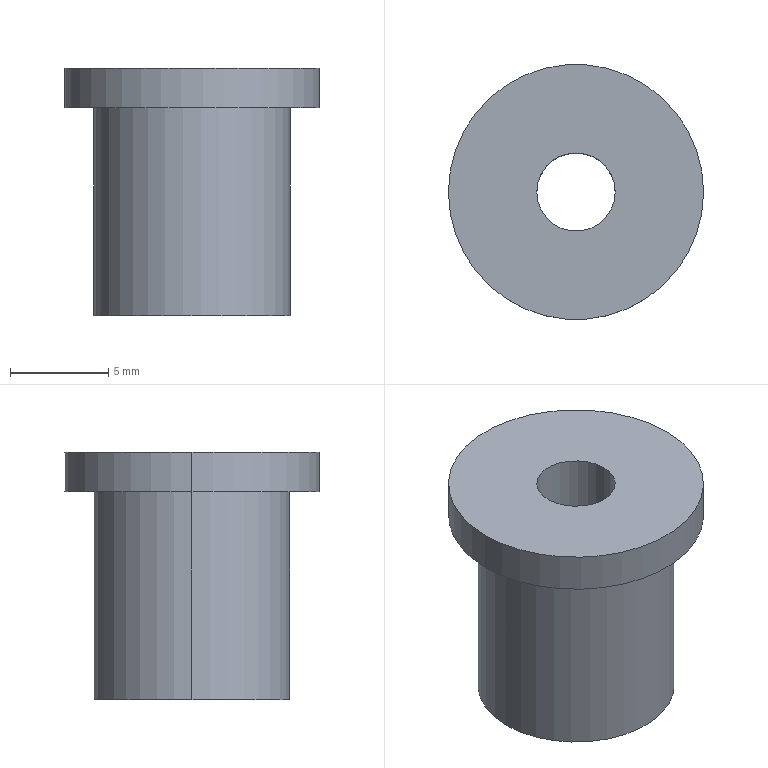Part | STEP file | 11-FG-B04011 | 1 solid | 9 faces | box 13 x 13 x 12.6 mm | volume 939.65 mm3 | cylinder 6 | plane 3 | commonest cylinder face diameters 4 x2 10 x2 13 x2
STEP:
#1=CARTESIAN_POINT('',(6.5,0.,12.6));
#2=VERTEX_POINT('',#1);
#3=CARTESIAN_POINT('',(-6.5,0.,12.6));
#4=VERTEX_POINT('',#3);
#5=CARTESIAN_POINT('',(0.,0.,12.6));
#6=DIRECTION('',(0.,0.,1.));
#7=DIRECTION('',(1.,0.,0.));
#8=AXIS2_PLACEMENT_3D('',#5,#6,#7);
#9=CIRCLE('',#8,6.5);
#10=EDGE_CURVE('',#2,#4,#9,.T.);
#11=ORIENTED_EDGE('',*,*,#10,.F.);
#12=CARTESIAN_POINT('',(6.5,0.,10.6));
#13=VERTEX_POINT('',#12);
#14=CARTESIAN_POINT('',(6.5,0.,12.6));
#15=DIRECTION('',(0.,0.,-1.));
#16=VECTOR('',#15,1000.);
#17=LINE('',#14,#16);
#18=EDGE_CURVE('',#2,#13,#17,.T.);
#19=ORIENTED_EDGE('',*,*,#18,.T.);
#20=CARTESIAN_POINT('',(-6.5,0.,10.6));
#21=VERTEX_POINT('',#20);
#22=CARTESIAN_POINT('',(0.,0.,10.6));
#23=DIRECTION('',(0.,0.,1.));
#24=DIRECTION('',(1.,0.,0.));
#25=AXIS2_PLACEMENT_3D('',#22,#23,#24);
#26=CIRCLE('',#25,6.5);
#27=EDGE_CURVE('',#13,#21,#26,.T.);
#28=ORIENTED_EDGE('',*,*,#27,.T.);
#29=CARTESIAN_POINT('',(-6.5,0.,12.6));
#30=DIRECTION('',(0.,0.,-1.));
#31=VECTOR('',#30,1000.);
#32=LINE('',#29,#31);
#33=EDGE_CURVE('',#4,#21,#32,.T.);
#34=ORIENTED_EDGE('',*,*,#33,.F.);
#35=EDGE_LOOP('',(#11,#19,#28,#34));
#36=FACE_OUTER_BOUND('',#35,.T.);
#37=CARTESIAN_POINT('',(0.,0.,12.6));
#38=DIRECTION('',(0.,0.,-1.));
#39=DIRECTION('',(-1.,0.,0.));
#40=AXIS2_PLACEMENT_3D('',#37,#38,#39);
#41=CYLINDRICAL_SURFACE('',#40,6.5);
#42=ADVANCED_FACE('',(#36),#41,.T.);
#43=CARTESIAN_POINT('',(-2.,0.,12.6));
#44=VERTEX_POINT('',#43);
#45=CARTESIAN_POINT('',(2.,0.,12.6));
#46=VERTEX_POINT('',#45);
#47=CARTESIAN_POINT('',(0.,0.,12.6));
#48=DIRECTION('',(0.,0.,1.));
#49=DIRECTION('',(1.,0.,0.));
#50=AXIS2_PLACEMENT_3D('',#47,#48,#49);
#51=CIRCLE('',#50,2.);
#52=EDGE_CURVE('',#44,#46,#51,.T.);
#53=ORIENTED_EDGE('',*,*,#52,.T.);
#54=CARTESIAN_POINT('',(2.,0.,0.));
#55=VERTEX_POINT('',#54);
#56=CARTESIAN_POINT('',(2.,0.,10.6));
#57=DIRECTION('',(0.,0.,-1.));
#58=VECTOR('',#57,1000.);
#59=LINE('',#56,#58);
#60=EDGE_CURVE('',#46,#55,#59,.T.);
#61=ORIENTED_EDGE('',*,*,#60,.T.);
#62=CARTESIAN_POINT('',(-2.,0.,0.));
#63=VERTEX_POINT('',#62);
#64=CARTESIAN_POINT('',(0.,0.,0.));
#65=DIRECTION('',(0.,0.,1.));
#66=DIRECTION('',(1.,0.,0.));
#67=AXIS2_PLACEMENT_3D('',#64,#65,#66);
#68=CIRCLE('',#67,2.);
#69=EDGE_CURVE('',#63,#55,#68,.T.);
#70=ORIENTED_EDGE('',*,*,#69,.F.);
#71=CARTESIAN_POINT('',(-2.,0.,10.6));
#72=DIRECTION('',(0.,0.,-1.));
#73=VECTOR('',#72,1000.);
#74=LINE('',#71,#73);
#75=EDGE_CURVE('',#44,#63,#74,.T.);
#76=ORIENTED_EDGE('',*,*,#75,.F.);
#77=EDGE_LOOP('',(#53,#61,#70,#76));
#78=FACE_OUTER_BOUND('',#77,.T.);
#79=CARTESIAN_POINT('',(0.,0.,10.6));
#80=DIRECTION('',(0.,0.,-1.));
#81=DIRECTION('',(-1.,0.,0.));
#82=AXIS2_PLACEMENT_3D('',#79,#80,#81);
#83=CYLINDRICAL_SURFACE('',#82,2.);
#84=ADVANCED_FACE('',(#78),#83,.F.);
#85=CARTESIAN_POINT('',(5.,0.,10.6));
#86=VERTEX_POINT('',#85);
#87=CARTESIAN_POINT('',(-5.,0.,10.6));
#88=VERTEX_POINT('',#87);
#89=CARTESIAN_POINT('',(0.,0.,10.6));
#90=DIRECTION('',(0.,0.,1.));
#91=DIRECTION('',(1.,0.,0.));
#92=AXIS2_PLACEMENT_3D('',#89,#90,#91);
#93=CIRCLE('',#92,5.);
#94=EDGE_CURVE('',#86,#88,#93,.T.);
#95=ORIENTED_EDGE('',*,*,#94,.F.);
#96=CARTESIAN_POINT('',(5.,0.,0.));
#97=VERTEX_POINT('',#96);
#98=CARTESIAN_POINT('',(5.,0.,10.6));
#99=DIRECTION('',(0.,0.,-1.));
#100=VECTOR('',#99,1000.);
#101=LINE('',#98,#100);
#102=EDGE_CURVE('',#86,#97,#101,.T.);
#103=ORIENTED_EDGE('',*,*,#102,.T.);
#104=CARTESIAN_POINT('',(-5.,0.,0.));
#105=VERTEX_POINT('',#104);
#106=CARTESIAN_POINT('',(0.,0.,0.));
#107=DIRECTION('',(0.,0.,1.));
#108=DIRECTION('',(1.,0.,0.));
#109=AXIS2_PLACEMENT_3D('',#106,#107,#108);
#110=CIRCLE('',#109,5.);
#111=EDGE_CURVE('',#97,#105,#110,.T.);
#112=ORIENTED_EDGE('',*,*,#111,.T.);
#113=CARTESIAN_POINT('',(-5.,0.,10.6));
#114=DIRECTION('',(0.,0.,-1.));
#115=VECTOR('',#114,1000.);
#116=LINE('',#113,#115);
#117=EDGE_CURVE('',#88,#105,#116,.T.);
#118=ORIENTED_EDGE('',*,*,#117,.F.);
#119=EDGE_LOOP('',(#95,#103,#112,#118));
#120=FACE_OUTER_BOUND('',#119,.T.);
#121=CARTESIAN_POINT('',(0.,0.,10.6));
#122=DIRECTION('',(0.,0.,-1.));
#123=DIRECTION('',(-1.,0.,0.));
#124=AXIS2_PLACEMENT_3D('',#121,#122,#123);
#125=CYLINDRICAL_SURFACE('',#124,5.);
#126=ADVANCED_FACE('',(#120),#125,.T.);
#127=CARTESIAN_POINT('',(0.,0.,0.));
#128=DIRECTION('',(0.,0.,1.));
#129=DIRECTION('',(1.,0.,0.));
#130=AXIS2_PLACEMENT_3D('',#127,#128,#129);
#131=CIRCLE('',#130,5.);
#132=EDGE_CURVE('',#105,#97,#131,.T.);
#133=ORIENTED_EDGE('',*,*,#132,.F.);
#134=ORIENTED_EDGE('',*,*,#111,.F.);
#135=EDGE_LOOP('',(#133,#134));
#136=FACE_OUTER_BOUND('',#135,.T.);
#137=ORIENTED_EDGE('',*,*,#69,.T.);
#138=CARTESIAN_POINT('',(0.,0.,0.));
#139=DIRECTION('',(0.,0.,1.));
#140=DIRECTION('',(1.,0.,0.));
#141=AXIS2_PLACEMENT_3D('',#138,#139,#140);
#142=CIRCLE('',#141,2.);
#143=EDGE_CURVE('',#55,#63,#142,.T.);
#144=ORIENTED_EDGE('',*,*,#143,.T.);
#145=EDGE_LOOP('',(#137,#144));
#146=FACE_BOUND('',#145,.T.);
#147=CARTESIAN_POINT('',(0.,0.,0.));
#148=DIRECTION('',(0.,0.,1.));
#149=DIRECTION('',(1.,0.,0.));
#150=AXIS2_PLACEMENT_3D('',#147,#148,#149);
#151=PLANE('',#150);
#152=ADVANCED_FACE('',(#136,#146),#151,.F.);
#153=ORIENTED_EDGE('',*,*,#102,.F.);
#154=CARTESIAN_POINT('',(0.,0.,10.6));
#155=DIRECTION('',(0.,0.,1.));
#156=DIRECTION('',(1.,0.,0.));
#157=AXIS2_PLACEMENT_3D('',#154,#155,#156);
#158=CIRCLE('',#157,5.);
#159=EDGE_CURVE('',#88,#86,#158,.T.);
#160=ORIENTED_EDGE('',*,*,#159,.F.);
#161=ORIENTED_EDGE('',*,*,#117,.T.);
#162=ORIENTED_EDGE('',*,*,#132,.T.);
#163=EDGE_LOOP('',(#153,#160,#161,#162));
#164=FACE_OUTER_BOUND('',#163,.T.);
#165=CARTESIAN_POINT('',(0.,0.,10.6));
#166=DIRECTION('',(0.,0.,-1.));
#167=DIRECTION('',(-1.,0.,0.));
#168=AXIS2_PLACEMENT_3D('',#165,#166,#167);
#169=CYLINDRICAL_SURFACE('',#168,5.);
#170=ADVANCED_FACE('',(#164),#169,.T.);
#171=ORIENTED_EDGE('',*,*,#60,.F.);
#172=CARTESIAN_POINT('',(0.,0.,12.6));
#173=DIRECTION('',(0.,0.,1.));
#174=DIRECTION('',(1.,0.,0.));
#175=AXIS2_PLACEMENT_3D('',#172,#173,#174);
#176=CIRCLE('',#175,2.);
#177=EDGE_CURVE('',#46,#44,#176,.T.);
#178=ORIENTED_EDGE('',*,*,#177,.T.);
#179=ORIENTED_EDGE('',*,*,#75,.T.);
#180=ORIENTED_EDGE('',*,*,#143,.F.);
#181=EDGE_LOOP('',(#171,#178,#179,#180));
#182=FACE_OUTER_BOUND('',#181,.T.);
#183=CARTESIAN_POINT('',(0.,0.,10.6));
#184=DIRECTION('',(0.,0.,-1.));
#185=DIRECTION('',(-1.,0.,0.));
#186=AXIS2_PLACEMENT_3D('',#183,#184,#185);
#187=CYLINDRICAL_SURFACE('',#186,2.);
#188=ADVANCED_FACE('',(#182),#187,.F.);
#189=CARTESIAN_POINT('',(0.,0.,10.6));
#190=DIRECTION('',(0.,0.,1.));
#191=DIRECTION('',(1.,0.,0.));
#192=AXIS2_PLACEMENT_3D('',#189,#190,#191);
#193=CIRCLE('',#192,6.5);
#194=EDGE_CURVE('',#21,#13,#193,.T.);
#195=ORIENTED_EDGE('',*,*,#194,.F.);
#196=ORIENTED_EDGE('',*,*,#27,.F.);
#197=EDGE_LOOP('',(#195,#196));
#198=FACE_OUTER_BOUND('',#197,.T.);
#199=ORIENTED_EDGE('',*,*,#159,.T.);
#200=ORIENTED_EDGE('',*,*,#94,.T.);
#201=EDGE_LOOP('',(#199,#200));
#202=FACE_BOUND('',#201,.T.);
#203=CARTESIAN_POINT('',(0.,0.,10.6));
#204=DIRECTION('',(0.,0.,1.));
#205=DIRECTION('',(1.,0.,0.));
#206=AXIS2_PLACEMENT_3D('',#203,#204,#205);
#207=PLANE('',#206);
#208=ADVANCED_FACE('',(#198,#202),#207,.F.);
#209=CARTESIAN_POINT('',(0.,0.,12.6));
#210=DIRECTION('',(0.,0.,1.));
#211=DIRECTION('',(1.,0.,0.));
#212=AXIS2_PLACEMENT_3D('',#209,#210,#211);
#213=CIRCLE('',#212,6.5);
#214=EDGE_CURVE('',#4,#2,#213,.T.);
#215=ORIENTED_EDGE('',*,*,#214,.T.);
#216=ORIENTED_EDGE('',*,*,#10,.T.);
#217=EDGE_LOOP('',(#215,#216));
#218=FACE_OUTER_BOUND('',#217,.T.);
#219=ORIENTED_EDGE('',*,*,#52,.F.);
#220=ORIENTED_EDGE('',*,*,#177,.F.);
#221=EDGE_LOOP('',(#219,#220));
#222=FACE_BOUND('',#221,.T.);
#223=CARTESIAN_POINT('',(0.,0.,12.6));
#224=DIRECTION('',(0.,0.,1.));
#225=DIRECTION('',(1.,0.,0.));
#226=AXIS2_PLACEMENT_3D('',#223,#224,#225);
#227=PLANE('',#226);
#228=ADVANCED_FACE('',(#218,#222),#227,.T.);
#229=ORIENTED_EDGE('',*,*,#18,.F.);
#230=ORIENTED_EDGE('',*,*,#214,.F.);
#231=ORIENTED_EDGE('',*,*,#33,.T.);
#232=ORIENTED_EDGE('',*,*,#194,.T.);
#233=EDGE_LOOP('',(#229,#230,#231,#232));
#234=FACE_OUTER_BOUND('',#233,.T.);
#235=CARTESIAN_POINT('',(0.,0.,12.6));
#236=DIRECTION('',(0.,0.,-1.));
#237=DIRECTION('',(-1.,0.,0.));
#238=AXIS2_PLACEMENT_3D('',#235,#236,#237);
#239=CYLINDRICAL_SURFACE('',#238,6.5);
#240=ADVANCED_FACE('',(#234),#239,.T.);
#241=CLOSED_SHELL('',(#42,#84,#126,#152,#170,#188,#208,#228,#240));
#242=MANIFOLD_SOLID_BREP('',#241);
#243=CARTESIAN_POINT('',(0.,0.,0.));
#244=DIRECTION('',(0.,0.,1.));
#245=DIRECTION('',(1.,0.,0.));
#246=AXIS2_PLACEMENT_3D('',#243,#244,#245);
#247=(LENGTH_UNIT()NAMED_UNIT(*)SI_UNIT(.MILLI.,.METRE.));
#248=UNCERTAINTY_MEASURE_WITH_UNIT(LENGTH_MEASURE(0.00001),#247,'','');
#249=(NAMED_UNIT(*)PLANE_ANGLE_UNIT()SI_UNIT($,.RADIAN.));
#250=(NAMED_UNIT(*)SI_UNIT($,.STERADIAN.)SOLID_ANGLE_UNIT());
#251=(GEOMETRIC_REPRESENTATION_CONTEXT(3)GLOBAL_UNCERTAINTY_ASSIGNED_CONTEXT((#248))GLOBAL_UNIT_ASSIGNED_CONTEXT((#247,#249,#250))REPRESENTATION_CONTEXT('',''));
#252=ADVANCED_BREP_SHAPE_REPRESENTATION('',(#242,#246),#251);